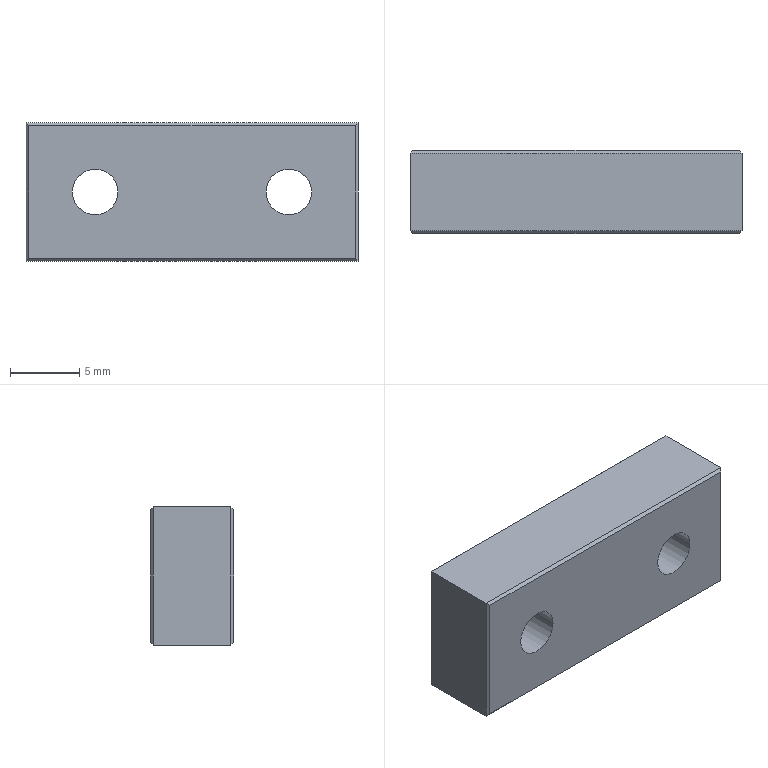Part | NX | 1 solid | 22 faces | box 24 x 6 x 10 mm | volume 1332 mm3 | plane 14 | cylinder 4 | cone 4 | commonest cylinder face diameters 3.3 x4
STEP:
#1=CARTESIAN_POINT('',(0.2,0.,-0.2));
#2=VERTEX_POINT('',#1);
#3=CARTESIAN_POINT('',(0.2,0.,-9.8));
#4=VERTEX_POINT('',#3);
#5=CARTESIAN_POINT('',(0.2,0.,0.));
#6=DIRECTION('',(0.,0.,-1.));
#7=VECTOR('',#6,1000.);
#8=LINE('',#5,#7);
#9=EDGE_CURVE('',#2,#4,#8,.T.);
#10=ORIENTED_EDGE('',*,*,#9,.T.);
#11=CARTESIAN_POINT('',(23.8,0.,-9.8));
#12=VERTEX_POINT('',#11);
#13=CARTESIAN_POINT('',(0.,0.,-9.8));
#14=DIRECTION('',(-1.,0.,0.));
#15=VECTOR('',#14,1000.);
#16=LINE('',#13,#15);
#17=EDGE_CURVE('',#12,#4,#16,.T.);
#18=ORIENTED_EDGE('',*,*,#17,.F.);
#19=CARTESIAN_POINT('',(23.8,0.,-0.2));
#20=VERTEX_POINT('',#19);
#21=CARTESIAN_POINT('',(23.8,0.,0.));
#22=DIRECTION('',(0.,0.,-1.));
#23=VECTOR('',#22,1000.);
#24=LINE('',#21,#23);
#25=EDGE_CURVE('',#20,#12,#24,.T.);
#26=ORIENTED_EDGE('',*,*,#25,.F.);
#27=CARTESIAN_POINT('',(0.,0.,-0.2));
#28=DIRECTION('',(1.,0.,0.));
#29=VECTOR('',#28,1000.);
#30=LINE('',#27,#29);
#31=EDGE_CURVE('',#2,#20,#30,.T.);
#32=ORIENTED_EDGE('',*,*,#31,.F.);
#33=EDGE_LOOP('',(#10,#18,#26,#32));
#34=FACE_BOUND('',#33,.T.);
#35=CARTESIAN_POINT('',(3.35,0.,-5.));
#36=VERTEX_POINT('',#35);
#37=CARTESIAN_POINT('',(6.65,0.,-5.));
#38=VERTEX_POINT('',#37);
#39=CARTESIAN_POINT('',(5.,0.,-5.));
#40=DIRECTION('',(0.,1.,0.));
#41=DIRECTION('',(1.,0.,0.));
#42=AXIS2_PLACEMENT_3D('',#39,#40,#41);
#43=CIRCLE('',#42,1.65);
#44=EDGE_CURVE('',#36,#38,#43,.T.);
#45=ORIENTED_EDGE('',*,*,#44,.T.);
#46=CARTESIAN_POINT('',(5.,0.,-5.));
#47=DIRECTION('',(0.,1.,0.));
#48=DIRECTION('',(1.,0.,0.));
#49=AXIS2_PLACEMENT_3D('',#46,#47,#48);
#50=CIRCLE('',#49,1.65);
#51=EDGE_CURVE('',#38,#36,#50,.T.);
#52=ORIENTED_EDGE('',*,*,#51,.T.);
#53=EDGE_LOOP('',(#45,#52));
#54=FACE_BOUND('',#53,.T.);
#55=CARTESIAN_POINT('',(20.65,0.,-5.));
#56=VERTEX_POINT('',#55);
#57=CARTESIAN_POINT('',(17.35,0.,-5.));
#58=VERTEX_POINT('',#57);
#59=CARTESIAN_POINT('',(19.,0.,-5.));
#60=DIRECTION('',(0.,1.,0.));
#61=DIRECTION('',(1.,0.,0.));
#62=AXIS2_PLACEMENT_3D('',#59,#60,#61);
#63=CIRCLE('',#62,1.65);
#64=EDGE_CURVE('',#56,#58,#63,.T.);
#65=ORIENTED_EDGE('',*,*,#64,.T.);
#66=CARTESIAN_POINT('',(19.,0.,-5.));
#67=DIRECTION('',(0.,1.,0.));
#68=DIRECTION('',(1.,0.,0.));
#69=AXIS2_PLACEMENT_3D('',#66,#67,#68);
#70=CIRCLE('',#69,1.65);
#71=EDGE_CURVE('',#58,#56,#70,.T.);
#72=ORIENTED_EDGE('',*,*,#71,.T.);
#73=EDGE_LOOP('',(#65,#72));
#74=FACE_BOUND('',#73,.T.);
#75=CARTESIAN_POINT('',(0.,0.,0.));
#76=DIRECTION('',(0.,1.,0.));
#77=DIRECTION('',(1.,0.,0.));
#78=AXIS2_PLACEMENT_3D('',#75,#76,#77);
#79=PLANE('',#78);
#80=ADVANCED_FACE('',(#34,#54,#74),#79,.F.);
#81=CARTESIAN_POINT('',(0.,5.8,0.));
#82=VERTEX_POINT('',#81);
#83=CARTESIAN_POINT('',(24.,5.8,0.));
#84=VERTEX_POINT('',#83);
#85=CARTESIAN_POINT('',(0.,5.8,0.));
#86=DIRECTION('',(1.,0.,0.));
#87=VECTOR('',#86,1000.);
#88=LINE('',#85,#87);
#89=EDGE_CURVE('',#82,#84,#88,.T.);
#90=ORIENTED_EDGE('',*,*,#89,.F.);
#91=CARTESIAN_POINT('',(0.,0.2,0.));
#92=VERTEX_POINT('',#91);
#93=CARTESIAN_POINT('',(0.,0.,0.));
#94=DIRECTION('',(0.,1.,0.));
#95=VECTOR('',#94,1000.);
#96=LINE('',#93,#95);
#97=EDGE_CURVE('',#92,#82,#96,.T.);
#98=ORIENTED_EDGE('',*,*,#97,.F.);
#99=CARTESIAN_POINT('',(24.,0.2,0.));
#100=VERTEX_POINT('',#99);
#101=CARTESIAN_POINT('',(0.,0.2,0.));
#102=DIRECTION('',(1.,0.,0.));
#103=VECTOR('',#102,1000.);
#104=LINE('',#101,#103);
#105=EDGE_CURVE('',#92,#100,#104,.T.);
#106=ORIENTED_EDGE('',*,*,#105,.T.);
#107=CARTESIAN_POINT('',(24.,0.,0.));
#108=DIRECTION('',(0.,1.,0.));
#109=VECTOR('',#108,1000.);
#110=LINE('',#107,#109);
#111=EDGE_CURVE('',#100,#84,#110,.T.);
#112=ORIENTED_EDGE('',*,*,#111,.T.);
#113=EDGE_LOOP('',(#90,#98,#106,#112));
#114=FACE_BOUND('',#113,.T.);
#115=CARTESIAN_POINT('',(0.,0.,0.));
#116=DIRECTION('',(0.,0.,1.));
#117=DIRECTION('',(1.,0.,0.));
#118=AXIS2_PLACEMENT_3D('',#115,#116,#117);
#119=PLANE('',#118);
#120=ADVANCED_FACE('',(#114),#119,.T.);
#121=CARTESIAN_POINT('',(0.,5.8,-10.));
#122=VERTEX_POINT('',#121);
#123=CARTESIAN_POINT('',(0.,5.8,0.));
#124=DIRECTION('',(0.,0.,1.));
#125=VECTOR('',#124,1000.);
#126=LINE('',#123,#125);
#127=EDGE_CURVE('',#122,#82,#126,.T.);
#128=ORIENTED_EDGE('',*,*,#127,.F.);
#129=CARTESIAN_POINT('',(0.,0.2,-10.));
#130=VERTEX_POINT('',#129);
#131=CARTESIAN_POINT('',(0.,0.,-10.));
#132=DIRECTION('',(0.,-1.,0.));
#133=VECTOR('',#132,1000.);
#134=LINE('',#131,#133);
#135=EDGE_CURVE('',#122,#130,#134,.T.);
#136=ORIENTED_EDGE('',*,*,#135,.T.);
#137=CARTESIAN_POINT('',(0.,0.2,0.));
#138=DIRECTION('',(0.,0.,-1.));
#139=VECTOR('',#138,1000.);
#140=LINE('',#137,#139);
#141=EDGE_CURVE('',#92,#130,#140,.T.);
#142=ORIENTED_EDGE('',*,*,#141,.F.);
#143=ORIENTED_EDGE('',*,*,#97,.T.);
#144=EDGE_LOOP('',(#128,#136,#142,#143));
#145=FACE_BOUND('',#144,.T.);
#146=CARTESIAN_POINT('',(0.,0.,-10.));
#147=DIRECTION('',(-1.,0.,0.));
#148=DIRECTION('',(0.,0.,1.));
#149=AXIS2_PLACEMENT_3D('',#146,#147,#148);
#150=PLANE('',#149);
#151=ADVANCED_FACE('',(#145),#150,.T.);
#152=CARTESIAN_POINT('',(24.,5.8,-10.));
#153=VERTEX_POINT('',#152);
#154=CARTESIAN_POINT('',(0.,5.8,-10.));
#155=DIRECTION('',(1.,0.,0.));
#156=VECTOR('',#155,1000.);
#157=LINE('',#154,#156);
#158=EDGE_CURVE('',#122,#153,#157,.T.);
#159=ORIENTED_EDGE('',*,*,#158,.T.);
#160=CARTESIAN_POINT('',(24.,0.2,-10.));
#161=VERTEX_POINT('',#160);
#162=CARTESIAN_POINT('',(24.,0.,-10.));
#163=DIRECTION('',(0.,-1.,0.));
#164=VECTOR('',#163,1000.);
#165=LINE('',#162,#164);
#166=EDGE_CURVE('',#153,#161,#165,.T.);
#167=ORIENTED_EDGE('',*,*,#166,.T.);
#168=CARTESIAN_POINT('',(0.,0.2,-10.));
#169=DIRECTION('',(-1.,0.,0.));
#170=VECTOR('',#169,1000.);
#171=LINE('',#168,#170);
#172=EDGE_CURVE('',#161,#130,#171,.T.);
#173=ORIENTED_EDGE('',*,*,#172,.T.);
#174=ORIENTED_EDGE('',*,*,#135,.F.);
#175=EDGE_LOOP('',(#159,#167,#173,#174));
#176=FACE_BOUND('',#175,.T.);
#177=CARTESIAN_POINT('',(10.,0.,-10.));
#178=DIRECTION('',(0.,0.,-1.));
#179=DIRECTION('',(0.,-1.,0.));
#180=AXIS2_PLACEMENT_3D('',#177,#178,#179);
#181=PLANE('',#180);
#182=ADVANCED_FACE('',(#176),#181,.T.);
#183=CARTESIAN_POINT('',(24.,5.8,0.));
#184=DIRECTION('',(0.,0.,-1.));
#185=VECTOR('',#184,1000.);
#186=LINE('',#183,#185);
#187=EDGE_CURVE('',#84,#153,#186,.T.);
#188=ORIENTED_EDGE('',*,*,#187,.F.);
#189=ORIENTED_EDGE('',*,*,#111,.F.);
#190=CARTESIAN_POINT('',(24.,0.2,0.));
#191=DIRECTION('',(0.,0.,1.));
#192=VECTOR('',#191,1000.);
#193=LINE('',#190,#192);
#194=EDGE_CURVE('',#161,#100,#193,.T.);
#195=ORIENTED_EDGE('',*,*,#194,.F.);
#196=ORIENTED_EDGE('',*,*,#166,.F.);
#197=EDGE_LOOP('',(#188,#189,#195,#196));
#198=FACE_BOUND('',#197,.T.);
#199=CARTESIAN_POINT('',(24.,0.,0.));
#200=DIRECTION('',(1.,0.,0.));
#201=DIRECTION('',(0.,1.,0.));
#202=AXIS2_PLACEMENT_3D('',#199,#200,#201);
#203=PLANE('',#202);
#204=ADVANCED_FACE('',(#198),#203,.T.);
#205=CARTESIAN_POINT('',(0.2,6.,-0.2));
#206=VERTEX_POINT('',#205);
#207=CARTESIAN_POINT('',(23.8,6.,-0.2));
#208=VERTEX_POINT('',#207);
#209=CARTESIAN_POINT('',(0.,6.,-0.2));
#210=DIRECTION('',(1.,0.,0.));
#211=VECTOR('',#210,1000.);
#212=LINE('',#209,#211);
#213=EDGE_CURVE('',#206,#208,#212,.T.);
#214=ORIENTED_EDGE('',*,*,#213,.T.);
#215=CARTESIAN_POINT('',(23.8,6.,-9.8));
#216=VERTEX_POINT('',#215);
#217=CARTESIAN_POINT('',(23.8,6.,0.));
#218=DIRECTION('',(0.,0.,-1.));
#219=VECTOR('',#218,1000.);
#220=LINE('',#217,#219);
#221=EDGE_CURVE('',#208,#216,#220,.T.);
#222=ORIENTED_EDGE('',*,*,#221,.T.);
#223=CARTESIAN_POINT('',(0.2,6.,-9.8));
#224=VERTEX_POINT('',#223);
#225=CARTESIAN_POINT('',(0.,6.,-9.8));
#226=DIRECTION('',(-1.,0.,0.));
#227=VECTOR('',#226,1000.);
#228=LINE('',#225,#227);
#229=EDGE_CURVE('',#216,#224,#228,.T.);
#230=ORIENTED_EDGE('',*,*,#229,.T.);
#231=CARTESIAN_POINT('',(0.2,6.,0.));
#232=DIRECTION('',(0.,0.,-1.));
#233=VECTOR('',#232,1000.);
#234=LINE('',#231,#233);
#235=EDGE_CURVE('',#206,#224,#234,.T.);
#236=ORIENTED_EDGE('',*,*,#235,.F.);
#237=EDGE_LOOP('',(#214,#222,#230,#236));
#238=FACE_BOUND('',#237,.T.);
#239=CARTESIAN_POINT('',(2.685,6.,-5.));
#240=VERTEX_POINT('',#239);
#241=CARTESIAN_POINT('',(7.315,6.,-5.));
#242=VERTEX_POINT('',#241);
#243=CARTESIAN_POINT('',(5.,6.,-5.));
#244=DIRECTION('',(0.,1.,0.));
#245=DIRECTION('',(1.,0.,0.));
#246=AXIS2_PLACEMENT_3D('',#243,#244,#245);
#247=CIRCLE('',#246,2.315);
#248=EDGE_CURVE('',#240,#242,#247,.T.);
#249=ORIENTED_EDGE('',*,*,#248,.F.);
#250=CARTESIAN_POINT('',(5.,6.,-5.));
#251=DIRECTION('',(0.,1.,0.));
#252=DIRECTION('',(1.,0.,0.));
#253=AXIS2_PLACEMENT_3D('',#250,#251,#252);
#254=CIRCLE('',#253,2.315);
#255=EDGE_CURVE('',#242,#240,#254,.T.);
#256=ORIENTED_EDGE('',*,*,#255,.F.);
#257=EDGE_LOOP('',(#249,#256));
#258=FACE_BOUND('',#257,.T.);
#259=CARTESIAN_POINT('',(16.685,6.,-5.));
#260=VERTEX_POINT('',#259);
#261=CARTESIAN_POINT('',(21.315,6.,-5.));
#262=VERTEX_POINT('',#261);
#263=CARTESIAN_POINT('',(19.,6.,-5.));
#264=DIRECTION('',(0.,1.,0.));
#265=DIRECTION('',(1.,0.,0.));
#266=AXIS2_PLACEMENT_3D('',#263,#264,#265);
#267=CIRCLE('',#266,2.315);
#268=EDGE_CURVE('',#260,#262,#267,.T.);
#269=ORIENTED_EDGE('',*,*,#268,.F.);
#270=CARTESIAN_POINT('',(19.,6.,-5.));
#271=DIRECTION('',(0.,1.,0.));
#272=DIRECTION('',(1.,0.,0.));
#273=AXIS2_PLACEMENT_3D('',#270,#271,#272);
#274=CIRCLE('',#273,2.315);
#275=EDGE_CURVE('',#262,#260,#274,.T.);
#276=ORIENTED_EDGE('',*,*,#275,.F.);
#277=EDGE_LOOP('',(#269,#276));
#278=FACE_BOUND('',#277,.T.);
#279=CARTESIAN_POINT('',(0.,6.,0.));
#280=DIRECTION('',(0.,1.,0.));
#281=DIRECTION('',(1.,0.,0.));
#282=AXIS2_PLACEMENT_3D('',#279,#280,#281);
#283=PLANE('',#282);
#284=ADVANCED_FACE('',(#238,#258,#278),#283,.T.);
#285=CARTESIAN_POINT('',(6.65,5.616,-5.));
#286=VERTEX_POINT('',#285);
#287=CARTESIAN_POINT('',(3.35,5.616,-5.));
#288=VERTEX_POINT('',#287);
#289=CARTESIAN_POINT('',(5.,5.616,-5.));
#290=DIRECTION('',(0.,1.,0.));
#291=DIRECTION('',(1.,0.,0.));
#292=AXIS2_PLACEMENT_3D('',#289,#290,#291);
#293=CIRCLE('',#292,1.65);
#294=EDGE_CURVE('',#286,#288,#293,.T.);
#295=ORIENTED_EDGE('',*,*,#294,.T.);
#296=CARTESIAN_POINT('',(3.35,6.,-5.));
#297=DIRECTION('',(0.,1.,0.));
#298=VECTOR('',#297,1000.);
#299=LINE('',#296,#298);
#300=EDGE_CURVE('',#288,#36,#299,.F.);
#301=ORIENTED_EDGE('',*,*,#300,.T.);
#302=ORIENTED_EDGE('',*,*,#51,.F.);
#303=CARTESIAN_POINT('',(6.65,6.,-5.));
#304=DIRECTION('',(0.,1.,0.));
#305=VECTOR('',#304,1000.);
#306=LINE('',#303,#305);
#307=EDGE_CURVE('',#286,#38,#306,.F.);
#308=ORIENTED_EDGE('',*,*,#307,.F.);
#309=EDGE_LOOP('',(#295,#301,#302,#308));
#310=FACE_BOUND('',#309,.T.);
#311=CARTESIAN_POINT('',(5.,6.,-5.));
#312=DIRECTION('',(0.,1.,0.));
#313=DIRECTION('',(1.,0.,0.));
#314=AXIS2_PLACEMENT_3D('',#311,#312,#313);
#315=CYLINDRICAL_SURFACE('',#314,1.65);
#316=ADVANCED_FACE('',(#310),#315,.F.);
#317=ORIENTED_EDGE('',*,*,#294,.F.);
#318=CARTESIAN_POINT('',(6.65,5.616,-5.));
#319=DIRECTION('',(0.866,0.5,0.));
#320=VECTOR('',#319,1000.);
#321=LINE('',#318,#320);
#322=EDGE_CURVE('',#286,#242,#321,.T.);
#323=ORIENTED_EDGE('',*,*,#322,.T.);
#324=ORIENTED_EDGE('',*,*,#255,.T.);
#325=CARTESIAN_POINT('',(3.35,5.616,-5.));
#326=DIRECTION('',(-0.866,0.5,0.));
#327=VECTOR('',#326,1000.);
#328=LINE('',#325,#327);
#329=EDGE_CURVE('',#288,#240,#328,.T.);
#330=ORIENTED_EDGE('',*,*,#329,.F.);
#331=EDGE_LOOP('',(#317,#323,#324,#330));
#332=FACE_BOUND('',#331,.T.);
#333=CARTESIAN_POINT('',(5.,5.616,-5.));
#334=DIRECTION('',(0.,1.,0.));
#335=DIRECTION('',(1.,0.,0.));
#336=AXIS2_PLACEMENT_3D('',#333,#334,#335);
#337=CONICAL_SURFACE('',#336,1.65,1.047);
#338=ADVANCED_FACE('',(#332),#337,.F.);
#339=ORIENTED_EDGE('',*,*,#17,.T.);
#340=CARTESIAN_POINT('',(0.2,0.,-9.8));
#341=DIRECTION('',(0.5774,-0.5774,0.5774));
#342=VECTOR('',#341,1000.);
#343=LINE('',#340,#342);
#344=EDGE_CURVE('',#130,#4,#343,.T.);
#345=ORIENTED_EDGE('',*,*,#344,.F.);
#346=ORIENTED_EDGE('',*,*,#172,.F.);
#347=CARTESIAN_POINT('',(23.8,0.,-9.8));
#348=DIRECTION('',(-0.5774,-0.5774,0.5774));
#349=VECTOR('',#348,1000.);
#350=LINE('',#347,#349);
#351=EDGE_CURVE('',#161,#12,#350,.T.);
#352=ORIENTED_EDGE('',*,*,#351,.T.);
#353=EDGE_LOOP('',(#339,#345,#346,#352));
#354=FACE_BOUND('',#353,.T.);
#355=CARTESIAN_POINT('',(5.,0.1,-9.9));
#356=DIRECTION('',(0.,-0.7071,-0.7071));
#357=DIRECTION('',(0.,-0.7071,0.7071));
#358=AXIS2_PLACEMENT_3D('',#355,#356,#357);
#359=PLANE('',#358);
#360=ADVANCED_FACE('',(#354),#359,.T.);
#361=ORIENTED_EDGE('',*,*,#25,.T.);
#362=ORIENTED_EDGE('',*,*,#351,.F.);
#363=ORIENTED_EDGE('',*,*,#194,.T.);
#364=CARTESIAN_POINT('',(24.,0.2,0.));
#365=DIRECTION('',(-0.5774,-0.5774,-0.5774));
#366=VECTOR('',#365,1000.);
#367=LINE('',#364,#366);
#368=EDGE_CURVE('',#100,#20,#367,.T.);
#369=ORIENTED_EDGE('',*,*,#368,.T.);
#370=EDGE_LOOP('',(#361,#362,#363,#369));
#371=FACE_BOUND('',#370,.T.);
#372=CARTESIAN_POINT('',(23.9,0.1,-5.));
#373=DIRECTION('',(0.7071,-0.7071,0.));
#374=DIRECTION('',(0.,0.,-1.));
#375=AXIS2_PLACEMENT_3D('',#372,#373,#374);
#376=PLANE('',#375);
#377=ADVANCED_FACE('',(#371),#376,.T.);
#378=ORIENTED_EDGE('',*,*,#31,.T.);
#379=ORIENTED_EDGE('',*,*,#368,.F.);
#380=ORIENTED_EDGE('',*,*,#105,.F.);
#381=CARTESIAN_POINT('',(0.,0.2,0.));
#382=DIRECTION('',(-0.5774,0.5774,0.5774));
#383=VECTOR('',#382,1000.);
#384=LINE('',#381,#383);
#385=EDGE_CURVE('',#2,#92,#384,.T.);
#386=ORIENTED_EDGE('',*,*,#385,.F.);
#387=EDGE_LOOP('',(#378,#379,#380,#386));
#388=FACE_BOUND('',#387,.T.);
#389=CARTESIAN_POINT('',(5.,0.1,-0.1));
#390=DIRECTION('',(0.,-0.7071,0.7071));
#391=DIRECTION('',(-1.,0.,0.));
#392=AXIS2_PLACEMENT_3D('',#389,#390,#391);
#393=PLANE('',#392);
#394=ADVANCED_FACE('',(#388),#393,.T.);
#395=ORIENTED_EDGE('',*,*,#9,.F.);
#396=ORIENTED_EDGE('',*,*,#385,.T.);
#397=ORIENTED_EDGE('',*,*,#141,.T.);
#398=ORIENTED_EDGE('',*,*,#344,.T.);
#399=EDGE_LOOP('',(#395,#396,#397,#398));
#400=FACE_BOUND('',#399,.T.);
#401=CARTESIAN_POINT('',(0.1,0.1,-5.));
#402=DIRECTION('',(-0.7071,-0.7071,0.));
#403=DIRECTION('',(-0.7071,0.7071,0.));
#404=AXIS2_PLACEMENT_3D('',#401,#402,#403);
#405=PLANE('',#404);
#406=ADVANCED_FACE('',(#400),#405,.T.);
#407=ORIENTED_EDGE('',*,*,#127,.T.);
#408=CARTESIAN_POINT('',(-5.8,0.,5.8));
#409=DIRECTION('',(0.5774,0.5774,-0.5774));
#410=VECTOR('',#409,1000.);
#411=LINE('',#408,#410);
#412=EDGE_CURVE('',#82,#206,#411,.T.);
#413=ORIENTED_EDGE('',*,*,#412,.T.);
#414=ORIENTED_EDGE('',*,*,#235,.T.);
#415=CARTESIAN_POINT('',(-5.8,0.,-15.8));
#416=DIRECTION('',(-0.5774,-0.5774,-0.5774));
#417=VECTOR('',#416,1000.);
#418=LINE('',#415,#417);
#419=EDGE_CURVE('',#224,#122,#418,.T.);
#420=ORIENTED_EDGE('',*,*,#419,.T.);
#421=EDGE_LOOP('',(#407,#413,#414,#420));
#422=FACE_BOUND('',#421,.T.);
#423=CARTESIAN_POINT('',(0.1,5.9,-5.));
#424=DIRECTION('',(-0.7071,0.7071,0.));
#425=DIRECTION('',(0.,0.,1.));
#426=AXIS2_PLACEMENT_3D('',#423,#424,#425);
#427=PLANE('',#426);
#428=ADVANCED_FACE('',(#422),#427,.T.);
#429=ORIENTED_EDGE('',*,*,#187,.T.);
#430=CARTESIAN_POINT('',(29.8,0.,-15.8));
#431=DIRECTION('',(0.5774,-0.5774,-0.5774));
#432=VECTOR('',#431,1000.);
#433=LINE('',#430,#432);
#434=EDGE_CURVE('',#216,#153,#433,.T.);
#435=ORIENTED_EDGE('',*,*,#434,.F.);
#436=ORIENTED_EDGE('',*,*,#221,.F.);
#437=CARTESIAN_POINT('',(29.8,0.,5.8));
#438=DIRECTION('',(0.5774,-0.5774,0.5774));
#439=VECTOR('',#438,1000.);
#440=LINE('',#437,#439);
#441=EDGE_CURVE('',#208,#84,#440,.T.);
#442=ORIENTED_EDGE('',*,*,#441,.T.);
#443=EDGE_LOOP('',(#429,#435,#436,#442));
#444=FACE_BOUND('',#443,.T.);
#445=CARTESIAN_POINT('',(23.9,5.9,-5.));
#446=DIRECTION('',(0.7071,0.7071,0.));
#447=DIRECTION('',(0.,0.,-1.));
#448=AXIS2_PLACEMENT_3D('',#445,#446,#447);
#449=PLANE('',#448);
#450=ADVANCED_FACE('',(#444),#449,.T.);
#451=ORIENTED_EDGE('',*,*,#89,.T.);
#452=ORIENTED_EDGE('',*,*,#441,.F.);
#453=ORIENTED_EDGE('',*,*,#213,.F.);
#454=ORIENTED_EDGE('',*,*,#412,.F.);
#455=EDGE_LOOP('',(#451,#452,#453,#454));
#456=FACE_BOUND('',#455,.T.);
#457=CARTESIAN_POINT('',(5.,5.9,-0.1));
#458=DIRECTION('',(0.,0.7071,0.7071));
#459=DIRECTION('',(1.,0.,0.));
#460=AXIS2_PLACEMENT_3D('',#457,#458,#459);
#461=PLANE('',#460);
#462=ADVANCED_FACE('',(#456),#461,.T.);
#463=ORIENTED_EDGE('',*,*,#158,.F.);
#464=ORIENTED_EDGE('',*,*,#419,.F.);
#465=ORIENTED_EDGE('',*,*,#229,.F.);
#466=ORIENTED_EDGE('',*,*,#434,.T.);
#467=EDGE_LOOP('',(#463,#464,#465,#466));
#468=FACE_BOUND('',#467,.T.);
#469=CARTESIAN_POINT('',(5.,5.9,-9.9));
#470=DIRECTION('',(0.,0.7071,-0.7071));
#471=DIRECTION('',(-1.,0.,0.));
#472=AXIS2_PLACEMENT_3D('',#469,#470,#471);
#473=PLANE('',#472);
#474=ADVANCED_FACE('',(#468),#473,.T.);
#475=ORIENTED_EDGE('',*,*,#64,.F.);
#476=CARTESIAN_POINT('',(20.65,5.616,-5.));
#477=VERTEX_POINT('',#476);
#478=CARTESIAN_POINT('',(20.65,6.,-5.));
#479=DIRECTION('',(0.,1.,0.));
#480=VECTOR('',#479,1000.);
#481=LINE('',#478,#480);
#482=EDGE_CURVE('',#56,#477,#481,.T.);
#483=ORIENTED_EDGE('',*,*,#482,.T.);
#484=CARTESIAN_POINT('',(17.35,5.616,-5.));
#485=VERTEX_POINT('',#484);
#486=CARTESIAN_POINT('',(19.,5.616,-5.));
#487=DIRECTION('',(0.,1.,0.));
#488=DIRECTION('',(1.,0.,0.));
#489=AXIS2_PLACEMENT_3D('',#486,#487,#488);
#490=CIRCLE('',#489,1.65);
#491=EDGE_CURVE('',#477,#485,#490,.T.);
#492=ORIENTED_EDGE('',*,*,#491,.T.);
#493=CARTESIAN_POINT('',(17.35,6.,-5.));
#494=DIRECTION('',(0.,1.,0.));
#495=VECTOR('',#494,1000.);
#496=LINE('',#493,#495);
#497=EDGE_CURVE('',#58,#485,#496,.T.);
#498=ORIENTED_EDGE('',*,*,#497,.F.);
#499=EDGE_LOOP('',(#475,#483,#492,#498));
#500=FACE_BOUND('',#499,.T.);
#501=CARTESIAN_POINT('',(19.,6.,-5.));
#502=DIRECTION('',(0.,1.,0.));
#503=DIRECTION('',(1.,0.,0.));
#504=AXIS2_PLACEMENT_3D('',#501,#502,#503);
#505=CYLINDRICAL_SURFACE('',#504,1.65);
#506=ADVANCED_FACE('',(#500),#505,.F.);
#507=CARTESIAN_POINT('',(19.,5.616,-5.));
#508=DIRECTION('',(0.,1.,0.));
#509=DIRECTION('',(1.,0.,0.));
#510=AXIS2_PLACEMENT_3D('',#507,#508,#509);
#511=CIRCLE('',#510,1.65);
#512=EDGE_CURVE('',#485,#477,#511,.T.);
#513=ORIENTED_EDGE('',*,*,#512,.F.);
#514=CARTESIAN_POINT('',(17.35,5.616,-5.));
#515=DIRECTION('',(-0.866,0.5,0.));
#516=VECTOR('',#515,1000.);
#517=LINE('',#514,#516);
#518=EDGE_CURVE('',#485,#260,#517,.T.);
#519=ORIENTED_EDGE('',*,*,#518,.T.);
#520=ORIENTED_EDGE('',*,*,#268,.T.);
#521=CARTESIAN_POINT('',(20.65,5.616,-5.));
#522=DIRECTION('',(0.866,0.5,0.));
#523=VECTOR('',#522,1000.);
#524=LINE('',#521,#523);
#525=EDGE_CURVE('',#477,#262,#524,.T.);
#526=ORIENTED_EDGE('',*,*,#525,.F.);
#527=EDGE_LOOP('',(#513,#519,#520,#526));
#528=FACE_BOUND('',#527,.T.);
#529=CARTESIAN_POINT('',(19.,5.616,-5.));
#530=DIRECTION('',(0.,1.,0.));
#531=DIRECTION('',(1.,0.,0.));
#532=AXIS2_PLACEMENT_3D('',#529,#530,#531);
#533=CONICAL_SURFACE('',#532,1.65,1.047);
#534=ADVANCED_FACE('',(#528),#533,.F.);
#535=ORIENTED_EDGE('',*,*,#248,.T.);
#536=ORIENTED_EDGE('',*,*,#322,.F.);
#537=CARTESIAN_POINT('',(5.,5.616,-5.));
#538=DIRECTION('',(0.,1.,0.));
#539=DIRECTION('',(1.,0.,0.));
#540=AXIS2_PLACEMENT_3D('',#537,#538,#539);
#541=CIRCLE('',#540,1.65);
#542=EDGE_CURVE('',#288,#286,#541,.T.);
#543=ORIENTED_EDGE('',*,*,#542,.F.);
#544=ORIENTED_EDGE('',*,*,#329,.T.);
#545=EDGE_LOOP('',(#535,#536,#543,#544));
#546=FACE_BOUND('',#545,.T.);
#547=CARTESIAN_POINT('',(5.,5.616,-5.));
#548=DIRECTION('',(0.,1.,0.));
#549=DIRECTION('',(1.,0.,0.));
#550=AXIS2_PLACEMENT_3D('',#547,#548,#549);
#551=CONICAL_SURFACE('',#550,1.65,1.047);
#552=ADVANCED_FACE('',(#546),#551,.F.);
#553=ORIENTED_EDGE('',*,*,#512,.T.);
#554=ORIENTED_EDGE('',*,*,#482,.F.);
#555=ORIENTED_EDGE('',*,*,#71,.F.);
#556=ORIENTED_EDGE('',*,*,#497,.T.);
#557=EDGE_LOOP('',(#553,#554,#555,#556));
#558=FACE_BOUND('',#557,.T.);
#559=CARTESIAN_POINT('',(19.,6.,-5.));
#560=DIRECTION('',(0.,1.,0.));
#561=DIRECTION('',(1.,0.,0.));
#562=AXIS2_PLACEMENT_3D('',#559,#560,#561);
#563=CYLINDRICAL_SURFACE('',#562,1.65);
#564=ADVANCED_FACE('',(#558),#563,.F.);
#565=ORIENTED_EDGE('',*,*,#525,.T.);
#566=ORIENTED_EDGE('',*,*,#275,.T.);
#567=ORIENTED_EDGE('',*,*,#518,.F.);
#568=ORIENTED_EDGE('',*,*,#491,.F.);
#569=EDGE_LOOP('',(#565,#566,#567,#568));
#570=FACE_BOUND('',#569,.T.);
#571=CARTESIAN_POINT('',(19.,5.616,-5.));
#572=DIRECTION('',(0.,1.,0.));
#573=DIRECTION('',(1.,0.,0.));
#574=AXIS2_PLACEMENT_3D('',#571,#572,#573);
#575=CONICAL_SURFACE('',#574,1.65,1.047);
#576=ADVANCED_FACE('',(#570),#575,.F.);
#577=ORIENTED_EDGE('',*,*,#44,.F.);
#578=ORIENTED_EDGE('',*,*,#300,.F.);
#579=ORIENTED_EDGE('',*,*,#542,.T.);
#580=ORIENTED_EDGE('',*,*,#307,.T.);
#581=EDGE_LOOP('',(#577,#578,#579,#580));
#582=FACE_BOUND('',#581,.T.);
#583=CARTESIAN_POINT('',(5.,6.,-5.));
#584=DIRECTION('',(0.,1.,0.));
#585=DIRECTION('',(1.,0.,0.));
#586=AXIS2_PLACEMENT_3D('',#583,#584,#585);
#587=CYLINDRICAL_SURFACE('',#586,1.65);
#588=ADVANCED_FACE('',(#582),#587,.F.);
#589=CLOSED_SHELL('',(#80,#120,#151,#182,#204,#284,#316,#338,#360,#377,#394,#406,#428,#450,#462,#474,#506,#534,#552,#564,#576,#588));
#590=MANIFOLD_SOLID_BREP('',#589);
#591=(LENGTH_UNIT()NAMED_UNIT(*)SI_UNIT(.MILLI.,.METRE.));
#592=UNCERTAINTY_MEASURE_WITH_UNIT(LENGTH_MEASURE(0.00001),#591,'','');
#593=(NAMED_UNIT(*)PLANE_ANGLE_UNIT()SI_UNIT($,.RADIAN.));
#594=(NAMED_UNIT(*)SI_UNIT($,.STERADIAN.)SOLID_ANGLE_UNIT());
#595=(GEOMETRIC_REPRESENTATION_CONTEXT(3)GLOBAL_UNCERTAINTY_ASSIGNED_CONTEXT((#592))GLOBAL_UNIT_ASSIGNED_CONTEXT((#591,#593,#594))REPRESENTATION_CONTEXT('',''));
#596=ADVANCED_BREP_SHAPE_REPRESENTATION('',(#590),#595);